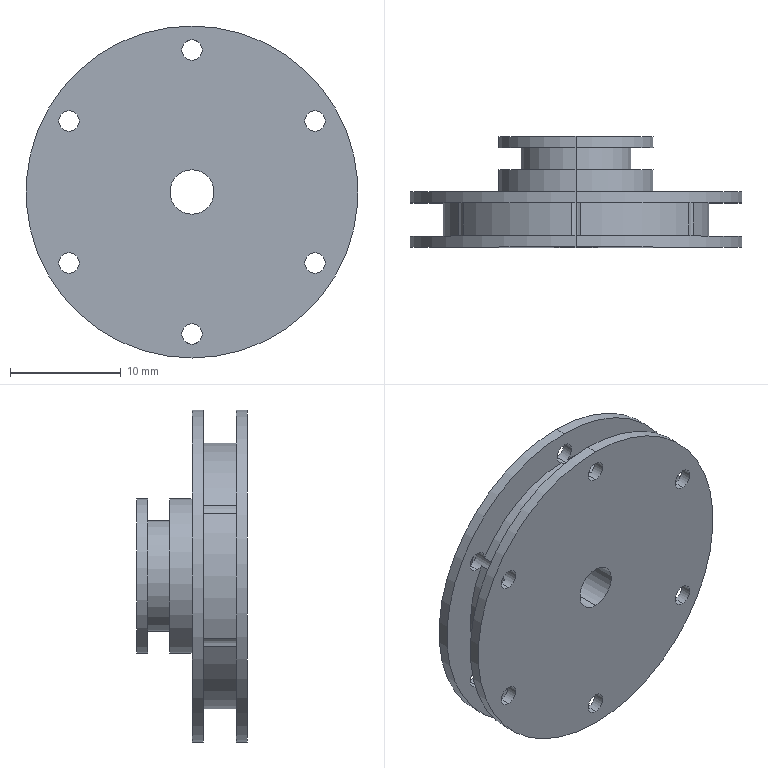Part | SolidWorks | features ICE 3, RevCut 2, Extrusion 1 | 1 solid | 41 faces | box 30 x 10 x 30 mm | volume 3231 mm3 | cylinder 34 | plane 7 | commonest cylinder face diameters 1.841 x16 24 x6 14 x4 30 x4 4 x2 10 x2